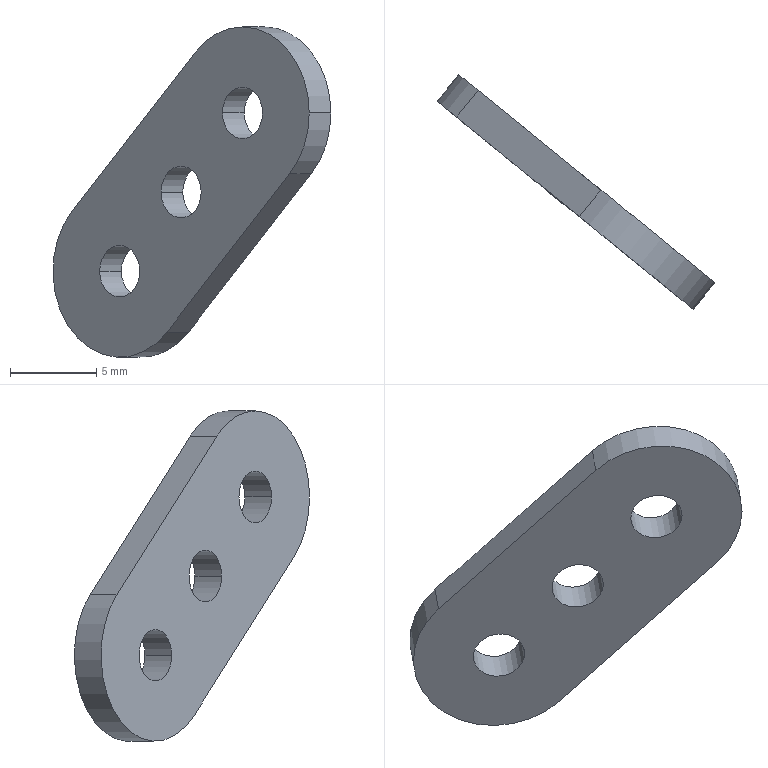Part | SolidWorks | features BaseBody 1 | 1 solid | 13 faces | box 16.152 x 13.661 x 19.192 mm | volume 374.668 mm3 | cylinder 9 | plane 4 | commonest cylinder face diameters 3 x6 10 x3
STEP:
#1=CARTESIAN_POINT('',(534.937,-167.759,275.623));
#2=VERTEX_POINT('',#1);
#3=CARTESIAN_POINT('',(536.073,-168.683,279.158));
#4=VERTEX_POINT('',#3);
#5=CARTESIAN_POINT('',(532.194,-165.528,279.158));
#6=DIRECTION('',(-0.6309,-0.7758,0.000000012));
#7=DIRECTION('',(0.7758,-0.6309,0.));
#8=AXIS2_PLACEMENT_3D('',#5,#6,#7);
#9=CIRCLE('',#8,5.);
#10=EDGE_CURVE('',#2,#4,#9,.T.);
#11=ORIENTED_EDGE('',*,*,#10,.T.);
#12=CARTESIAN_POINT('',(534.812,-170.235,279.158));
#13=VERTEX_POINT('',#12);
#14=CARTESIAN_POINT('',(536.073,-168.683,279.158));
#15=DIRECTION('',(-0.6309,-0.7758,0.000000012));
#16=VECTOR('',#15,1000.);
#17=LINE('',#14,#16);
#18=EDGE_CURVE('',#4,#13,#17,.T.);
#19=ORIENTED_EDGE('',*,*,#18,.T.);
#20=CARTESIAN_POINT('',(533.675,-169.311,275.623));
#21=VERTEX_POINT('',#20);
#22=CARTESIAN_POINT('',(530.932,-167.08,279.158));
#23=DIRECTION('',(0.6309,0.7758,-0.000000012));
#24=DIRECTION('',(0.7758,-0.6309,0.));
#25=AXIS2_PLACEMENT_3D('',#22,#23,#24);
#26=CIRCLE('',#25,5.);
#27=EDGE_CURVE('',#13,#21,#26,.T.);
#28=ORIENTED_EDGE('',*,*,#27,.T.);
#29=CARTESIAN_POINT('',(534.937,-167.759,275.623));
#30=DIRECTION('',(0.6309,0.7758,-0.000000012));
#31=VECTOR('',#30,1000.);
#32=LINE('',#29,#31);
#33=EDGE_CURVE('',#21,#2,#32,.T.);
#34=ORIENTED_EDGE('',*,*,#33,.T.);
#35=EDGE_LOOP('',(#11,#19,#28,#34));
#36=FACE_OUTER_BOUND('',#35,.T.);
#37=CARTESIAN_POINT('',(532.194,-165.528,279.158));
#38=DIRECTION('',(-0.6309,-0.7758,0.000000012));
#39=DIRECTION('',(0.7758,-0.6309,0.));
#40=AXIS2_PLACEMENT_3D('',#37,#38,#39);
#41=CYLINDRICAL_SURFACE('',#40,5.);
#42=ADVANCED_FACE('',(#36),#41,.T.);
#43=CARTESIAN_POINT('',(529.792,-163.575,274.562));
#44=VERTEX_POINT('',#43);
#45=CARTESIAN_POINT('',(527.465,-161.682,274.562));
#46=VERTEX_POINT('',#45);
#47=CARTESIAN_POINT('',(528.628,-162.628,274.562));
#48=DIRECTION('',(0.6309,0.7758,-0.000000012));
#49=DIRECTION('',(0.7758,-0.6309,0.));
#50=AXIS2_PLACEMENT_3D('',#47,#48,#49);
#51=CIRCLE('',#50,1.5);
#52=EDGE_CURVE('',#44,#46,#51,.T.);
#53=ORIENTED_EDGE('',*,*,#52,.T.);
#54=CARTESIAN_POINT('',(526.203,-163.234,274.562));
#55=VERTEX_POINT('',#54);
#56=CARTESIAN_POINT('',(526.203,-163.234,274.562));
#57=DIRECTION('',(-0.6309,-0.7758,0.000000012));
#58=VECTOR('',#57,1000.);
#59=LINE('',#56,#58);
#60=EDGE_CURVE('',#46,#55,#59,.T.);
#61=ORIENTED_EDGE('',*,*,#60,.T.);
#62=CARTESIAN_POINT('',(528.53,-165.127,274.562));
#63=VERTEX_POINT('',#62);
#64=CARTESIAN_POINT('',(527.366,-164.18,274.562));
#65=DIRECTION('',(0.6309,0.7758,-0.000000012));
#66=DIRECTION('',(0.7758,-0.6309,0.));
#67=AXIS2_PLACEMENT_3D('',#64,#65,#66);
#68=CIRCLE('',#67,1.5);
#69=EDGE_CURVE('',#63,#55,#68,.T.);
#70=ORIENTED_EDGE('',*,*,#69,.F.);
#71=CARTESIAN_POINT('',(528.53,-165.127,274.562));
#72=DIRECTION('',(-0.6309,-0.7758,0.000000012));
#73=VECTOR('',#72,1000.);
#74=LINE('',#71,#73);
#75=EDGE_CURVE('',#44,#63,#74,.T.);
#76=ORIENTED_EDGE('',*,*,#75,.F.);
#77=EDGE_LOOP('',(#53,#61,#70,#76));
#78=FACE_OUTER_BOUND('',#77,.T.);
#79=CARTESIAN_POINT('',(527.366,-164.18,274.562));
#80=DIRECTION('',(-0.6309,-0.7758,0.000000012));
#81=DIRECTION('',(0.7758,-0.6309,0.));
#82=AXIS2_PLACEMENT_3D('',#79,#80,#81);
#83=CYLINDRICAL_SURFACE('',#82,1.5);
#84=ADVANCED_FACE('',(#78),#83,.F.);
#85=CARTESIAN_POINT('',(526.226,-160.675,269.966));
#86=VERTEX_POINT('',#85);
#87=CARTESIAN_POINT('',(523.899,-158.782,269.966));
#88=VERTEX_POINT('',#87);
#89=CARTESIAN_POINT('',(525.062,-159.729,269.966));
#90=DIRECTION('',(0.6309,0.7758,-0.000000012));
#91=DIRECTION('',(0.7758,-0.6309,0.));
#92=AXIS2_PLACEMENT_3D('',#89,#90,#91);
#93=CIRCLE('',#92,1.5);
#94=EDGE_CURVE('',#86,#88,#93,.T.);
#95=ORIENTED_EDGE('',*,*,#94,.T.);
#96=CARTESIAN_POINT('',(522.637,-160.334,269.966));
#97=VERTEX_POINT('',#96);
#98=CARTESIAN_POINT('',(522.637,-160.334,269.966));
#99=DIRECTION('',(-0.6309,-0.7758,0.000000012));
#100=VECTOR('',#99,1000.);
#101=LINE('',#98,#100);
#102=EDGE_CURVE('',#88,#97,#101,.T.);
#103=ORIENTED_EDGE('',*,*,#102,.T.);
#104=CARTESIAN_POINT('',(524.964,-162.227,269.966));
#105=VERTEX_POINT('',#104);
#106=CARTESIAN_POINT('',(523.801,-161.28,269.966));
#107=DIRECTION('',(0.6309,0.7758,-0.000000012));
#108=DIRECTION('',(0.7758,-0.6309,0.));
#109=AXIS2_PLACEMENT_3D('',#106,#107,#108);
#110=CIRCLE('',#109,1.5);
#111=EDGE_CURVE('',#105,#97,#110,.T.);
#112=ORIENTED_EDGE('',*,*,#111,.F.);
#113=CARTESIAN_POINT('',(524.964,-162.227,269.966));
#114=DIRECTION('',(-0.6309,-0.7758,0.000000012));
#115=VECTOR('',#114,1000.);
#116=LINE('',#113,#115);
#117=EDGE_CURVE('',#86,#105,#116,.T.);
#118=ORIENTED_EDGE('',*,*,#117,.F.);
#119=EDGE_LOOP('',(#95,#103,#112,#118));
#120=FACE_OUTER_BOUND('',#119,.T.);
#121=CARTESIAN_POINT('',(523.801,-161.28,269.966));
#122=DIRECTION('',(-0.6309,-0.7758,0.000000012));
#123=DIRECTION('',(0.7758,-0.6309,0.));
#124=AXIS2_PLACEMENT_3D('',#121,#122,#123);
#125=CYLINDRICAL_SURFACE('',#124,1.5);
#126=ADVANCED_FACE('',(#120),#125,.F.);
#127=CARTESIAN_POINT('',(533.358,-166.475,279.158));
#128=VERTEX_POINT('',#127);
#129=CARTESIAN_POINT('',(531.03,-164.582,279.158));
#130=VERTEX_POINT('',#129);
#131=CARTESIAN_POINT('',(532.194,-165.528,279.158));
#132=DIRECTION('',(0.6309,0.7758,-0.000000012));
#133=DIRECTION('',(0.7758,-0.6309,0.));
#134=AXIS2_PLACEMENT_3D('',#131,#132,#133);
#135=CIRCLE('',#134,1.5);
#136=EDGE_CURVE('',#128,#130,#135,.T.);
#137=ORIENTED_EDGE('',*,*,#136,.T.);
#138=CARTESIAN_POINT('',(529.769,-166.134,279.158));
#139=VERTEX_POINT('',#138);
#140=CARTESIAN_POINT('',(529.769,-166.134,279.158));
#141=DIRECTION('',(-0.6309,-0.7758,0.000000012));
#142=VECTOR('',#141,1000.);
#143=LINE('',#140,#142);
#144=EDGE_CURVE('',#130,#139,#143,.T.);
#145=ORIENTED_EDGE('',*,*,#144,.T.);
#146=CARTESIAN_POINT('',(532.096,-168.026,279.158));
#147=VERTEX_POINT('',#146);
#148=CARTESIAN_POINT('',(530.932,-167.08,279.158));
#149=DIRECTION('',(0.6309,0.7758,-0.000000012));
#150=DIRECTION('',(0.7758,-0.6309,0.));
#151=AXIS2_PLACEMENT_3D('',#148,#149,#150);
#152=CIRCLE('',#151,1.5);
#153=EDGE_CURVE('',#147,#139,#152,.T.);
#154=ORIENTED_EDGE('',*,*,#153,.F.);
#155=CARTESIAN_POINT('',(532.096,-168.026,279.158));
#156=DIRECTION('',(-0.6309,-0.7758,0.000000012));
#157=VECTOR('',#156,1000.);
#158=LINE('',#155,#157);
#159=EDGE_CURVE('',#128,#147,#158,.T.);
#160=ORIENTED_EDGE('',*,*,#159,.F.);
#161=EDGE_LOOP('',(#137,#145,#154,#160));
#162=FACE_OUTER_BOUND('',#161,.T.);
#163=CARTESIAN_POINT('',(530.932,-167.08,279.158));
#164=DIRECTION('',(-0.6309,-0.7758,0.000000012));
#165=DIRECTION('',(0.7758,-0.6309,0.));
#166=AXIS2_PLACEMENT_3D('',#163,#164,#165);
#167=CYLINDRICAL_SURFACE('',#166,1.5);
#168=ADVANCED_FACE('',(#162),#167,.F.);
#169=CARTESIAN_POINT('',(527.805,-161.959,266.431));
#170=VERTEX_POINT('',#169);
#171=CARTESIAN_POINT('',(527.805,-161.959,266.431));
#172=DIRECTION('',(0.5486,-0.4461,0.7071));
#173=VECTOR('',#172,1000.);
#174=LINE('',#171,#173);
#175=EDGE_CURVE('',#170,#2,#174,.T.);
#176=ORIENTED_EDGE('',*,*,#175,.F.);
#177=CARTESIAN_POINT('',(522.319,-157.498,273.502));
#178=VERTEX_POINT('',#177);
#179=CARTESIAN_POINT('',(525.062,-159.729,269.966));
#180=DIRECTION('',(-0.6309,-0.7758,0.000000012));
#181=DIRECTION('',(0.7758,-0.6309,0.));
#182=AXIS2_PLACEMENT_3D('',#179,#180,#181);
#183=CIRCLE('',#182,5.);
#184=EDGE_CURVE('',#178,#170,#183,.T.);
#185=ORIENTED_EDGE('',*,*,#184,.F.);
#186=CARTESIAN_POINT('',(529.451,-163.298,282.694));
#187=VERTEX_POINT('',#186);
#188=CARTESIAN_POINT('',(529.451,-163.298,282.694));
#189=DIRECTION('',(-0.5486,0.4461,-0.7071));
#190=VECTOR('',#189,1000.);
#191=LINE('',#188,#190);
#192=EDGE_CURVE('',#187,#178,#191,.T.);
#193=ORIENTED_EDGE('',*,*,#192,.F.);
#194=CARTESIAN_POINT('',(532.194,-165.528,279.158));
#195=DIRECTION('',(-0.6309,-0.7758,0.000000012));
#196=DIRECTION('',(0.7758,-0.6309,0.));
#197=AXIS2_PLACEMENT_3D('',#194,#195,#196);
#198=CIRCLE('',#197,5.);
#199=EDGE_CURVE('',#4,#187,#198,.T.);
#200=ORIENTED_EDGE('',*,*,#199,.F.);
#201=ORIENTED_EDGE('',*,*,#10,.F.);
#202=EDGE_LOOP('',(#176,#185,#193,#200,#201));
#203=FACE_OUTER_BOUND('',#202,.T.);
#204=ORIENTED_EDGE('',*,*,#52,.F.);
#205=CARTESIAN_POINT('',(528.628,-162.628,274.562));
#206=DIRECTION('',(0.6309,0.7758,-0.000000012));
#207=DIRECTION('',(0.7758,-0.6309,0.));
#208=AXIS2_PLACEMENT_3D('',#205,#206,#207);
#209=CIRCLE('',#208,1.5);
#210=EDGE_CURVE('',#46,#44,#209,.T.);
#211=ORIENTED_EDGE('',*,*,#210,.F.);
#212=EDGE_LOOP('',(#204,#211));
#213=FACE_BOUND('',#212,.T.);
#214=ORIENTED_EDGE('',*,*,#94,.F.);
#215=CARTESIAN_POINT('',(525.062,-159.729,269.966));
#216=DIRECTION('',(0.6309,0.7758,-0.000000012));
#217=DIRECTION('',(0.7758,-0.6309,0.));
#218=AXIS2_PLACEMENT_3D('',#215,#216,#217);
#219=CIRCLE('',#218,1.5);
#220=EDGE_CURVE('',#88,#86,#219,.T.);
#221=ORIENTED_EDGE('',*,*,#220,.F.);
#222=EDGE_LOOP('',(#214,#221));
#223=FACE_BOUND('',#222,.T.);
#224=ORIENTED_EDGE('',*,*,#136,.F.);
#225=CARTESIAN_POINT('',(532.194,-165.528,279.158));
#226=DIRECTION('',(0.6309,0.7758,-0.000000012));
#227=DIRECTION('',(0.7758,-0.6309,0.));
#228=AXIS2_PLACEMENT_3D('',#225,#226,#227);
#229=CIRCLE('',#228,1.5);
#230=EDGE_CURVE('',#130,#128,#229,.T.);
#231=ORIENTED_EDGE('',*,*,#230,.F.);
#232=EDGE_LOOP('',(#224,#231));
#233=FACE_BOUND('',#232,.T.);
#234=CARTESIAN_POINT('',(528.628,-162.628,274.562));
#235=DIRECTION('',(-0.6309,-0.7758,0.000000012));
#236=DIRECTION('',(0.7758,-0.6309,0.));
#237=AXIS2_PLACEMENT_3D('',#234,#235,#236);
#238=PLANE('',#237);
#239=ADVANCED_FACE('',(#203,#213,#223,#233),#238,.F.);
#240=ORIENTED_EDGE('',*,*,#18,.F.);
#241=ORIENTED_EDGE('',*,*,#199,.T.);
#242=CARTESIAN_POINT('',(528.189,-164.849,282.694));
#243=VERTEX_POINT('',#242);
#244=CARTESIAN_POINT('',(528.189,-164.849,282.694));
#245=DIRECTION('',(0.6309,0.7758,-0.000000012));
#246=VECTOR('',#245,1000.);
#247=LINE('',#244,#246);
#248=EDGE_CURVE('',#243,#187,#247,.T.);
#249=ORIENTED_EDGE('',*,*,#248,.F.);
#250=CARTESIAN_POINT('',(530.932,-167.08,279.158));
#251=DIRECTION('',(0.6309,0.7758,-0.000000012));
#252=DIRECTION('',(0.7758,-0.6309,0.));
#253=AXIS2_PLACEMENT_3D('',#250,#251,#252);
#254=CIRCLE('',#253,5.);
#255=EDGE_CURVE('',#243,#13,#254,.T.);
#256=ORIENTED_EDGE('',*,*,#255,.T.);
#257=EDGE_LOOP('',(#240,#241,#249,#256));
#258=FACE_OUTER_BOUND('',#257,.T.);
#259=CARTESIAN_POINT('',(532.194,-165.528,279.158));
#260=DIRECTION('',(-0.6309,-0.7758,0.000000012));
#261=DIRECTION('',(0.7758,-0.6309,0.));
#262=AXIS2_PLACEMENT_3D('',#259,#260,#261);
#263=CYLINDRICAL_SURFACE('',#262,5.);
#264=ADVANCED_FACE('',(#258),#263,.T.);
#265=CARTESIAN_POINT('',(526.544,-163.511,266.431));
#266=VERTEX_POINT('',#265);
#267=CARTESIAN_POINT('',(526.544,-163.511,266.431));
#268=DIRECTION('',(0.6309,0.7758,-0.000000012));
#269=VECTOR('',#268,1000.);
#270=LINE('',#267,#269);
#271=EDGE_CURVE('',#266,#170,#270,.T.);
#272=ORIENTED_EDGE('',*,*,#271,.T.);
#273=ORIENTED_EDGE('',*,*,#175,.T.);
#274=ORIENTED_EDGE('',*,*,#33,.F.);
#275=CARTESIAN_POINT('',(533.675,-169.311,275.623));
#276=DIRECTION('',(-0.5486,0.4461,-0.7071));
#277=VECTOR('',#276,1000.);
#278=LINE('',#275,#277);
#279=EDGE_CURVE('',#21,#266,#278,.T.);
#280=ORIENTED_EDGE('',*,*,#279,.T.);
#281=EDGE_LOOP('',(#272,#273,#274,#280));
#282=FACE_OUTER_BOUND('',#281,.T.);
#283=CARTESIAN_POINT('',(537.68,-169.99,279.158));
#284=DIRECTION('',(0.5486,-0.4461,-0.7071));
#285=DIRECTION('',(-0.7901,0.,-0.613));
#286=AXIS2_PLACEMENT_3D('',#283,#284,#285);
#287=PLANE('',#286);
#288=ADVANCED_FACE('',(#282),#287,.T.);
#289=ORIENTED_EDGE('',*,*,#271,.F.);
#290=CARTESIAN_POINT('',(521.058,-159.05,273.502));
#291=VERTEX_POINT('',#290);
#292=CARTESIAN_POINT('',(523.801,-161.28,269.966));
#293=DIRECTION('',(0.6309,0.7758,-0.000000012));
#294=DIRECTION('',(0.7758,-0.6309,0.));
#295=AXIS2_PLACEMENT_3D('',#292,#293,#294);
#296=CIRCLE('',#295,5.);
#297=EDGE_CURVE('',#266,#291,#296,.T.);
#298=ORIENTED_EDGE('',*,*,#297,.T.);
#299=CARTESIAN_POINT('',(522.319,-157.498,273.502));
#300=DIRECTION('',(0.6309,0.7758,-0.000000012));
#301=VECTOR('',#300,1000.);
#302=LINE('',#299,#301);
#303=EDGE_CURVE('',#291,#178,#302,.T.);
#304=ORIENTED_EDGE('',*,*,#303,.T.);
#305=ORIENTED_EDGE('',*,*,#184,.T.);
#306=EDGE_LOOP('',(#289,#298,#304,#305));
#307=FACE_OUTER_BOUND('',#306,.T.);
#308=CARTESIAN_POINT('',(525.062,-159.729,269.966));
#309=DIRECTION('',(-0.6309,-0.7758,0.000000012));
#310=DIRECTION('',(0.7758,-0.6309,0.));
#311=AXIS2_PLACEMENT_3D('',#308,#309,#310);
#312=CYLINDRICAL_SURFACE('',#311,5.);
#313=ADVANCED_FACE('',(#307),#312,.T.);
#314=ORIENTED_EDGE('',*,*,#303,.F.);
#315=CARTESIAN_POINT('',(521.058,-159.05,273.502));
#316=DIRECTION('',(0.5486,-0.4461,0.7071));
#317=VECTOR('',#316,1000.);
#318=LINE('',#315,#317);
#319=EDGE_CURVE('',#291,#243,#318,.T.);
#320=ORIENTED_EDGE('',*,*,#319,.T.);
#321=ORIENTED_EDGE('',*,*,#248,.T.);
#322=ORIENTED_EDGE('',*,*,#192,.T.);
#323=EDGE_LOOP('',(#314,#320,#321,#322));
#324=FACE_OUTER_BOUND('',#323,.T.);
#325=CARTESIAN_POINT('',(519.576,-155.267,269.966));
#326=DIRECTION('',(-0.5486,0.4461,0.7071));
#327=DIRECTION('',(0.7901,0.,0.613));
#328=AXIS2_PLACEMENT_3D('',#325,#326,#327);
#329=PLANE('',#328);
#330=ADVANCED_FACE('',(#324),#329,.T.);
#331=ORIENTED_EDGE('',*,*,#60,.F.);
#332=ORIENTED_EDGE('',*,*,#210,.T.);
#333=ORIENTED_EDGE('',*,*,#75,.T.);
#334=CARTESIAN_POINT('',(527.366,-164.18,274.562));
#335=DIRECTION('',(0.6309,0.7758,-0.000000012));
#336=DIRECTION('',(0.7758,-0.6309,0.));
#337=AXIS2_PLACEMENT_3D('',#334,#335,#336);
#338=CIRCLE('',#337,1.5);
#339=EDGE_CURVE('',#55,#63,#338,.T.);
#340=ORIENTED_EDGE('',*,*,#339,.F.);
#341=EDGE_LOOP('',(#331,#332,#333,#340));
#342=FACE_OUTER_BOUND('',#341,.T.);
#343=CARTESIAN_POINT('',(527.366,-164.18,274.562));
#344=DIRECTION('',(-0.6309,-0.7758,0.000000012));
#345=DIRECTION('',(0.7758,-0.6309,0.));
#346=AXIS2_PLACEMENT_3D('',#343,#344,#345);
#347=CYLINDRICAL_SURFACE('',#346,1.5);
#348=ADVANCED_FACE('',(#342),#347,.F.);
#349=ORIENTED_EDGE('',*,*,#102,.F.);
#350=ORIENTED_EDGE('',*,*,#220,.T.);
#351=ORIENTED_EDGE('',*,*,#117,.T.);
#352=CARTESIAN_POINT('',(523.801,-161.28,269.966));
#353=DIRECTION('',(0.6309,0.7758,-0.000000012));
#354=DIRECTION('',(0.7758,-0.6309,0.));
#355=AXIS2_PLACEMENT_3D('',#352,#353,#354);
#356=CIRCLE('',#355,1.5);
#357=EDGE_CURVE('',#97,#105,#356,.T.);
#358=ORIENTED_EDGE('',*,*,#357,.F.);
#359=EDGE_LOOP('',(#349,#350,#351,#358));
#360=FACE_OUTER_BOUND('',#359,.T.);
#361=CARTESIAN_POINT('',(523.801,-161.28,269.966));
#362=DIRECTION('',(-0.6309,-0.7758,0.000000012));
#363=DIRECTION('',(0.7758,-0.6309,0.));
#364=AXIS2_PLACEMENT_3D('',#361,#362,#363);
#365=CYLINDRICAL_SURFACE('',#364,1.5);
#366=ADVANCED_FACE('',(#360),#365,.F.);
#367=ORIENTED_EDGE('',*,*,#144,.F.);
#368=ORIENTED_EDGE('',*,*,#230,.T.);
#369=ORIENTED_EDGE('',*,*,#159,.T.);
#370=CARTESIAN_POINT('',(530.932,-167.08,279.158));
#371=DIRECTION('',(0.6309,0.7758,-0.000000012));
#372=DIRECTION('',(0.7758,-0.6309,0.));
#373=AXIS2_PLACEMENT_3D('',#370,#371,#372);
#374=CIRCLE('',#373,1.5);
#375=EDGE_CURVE('',#139,#147,#374,.T.);
#376=ORIENTED_EDGE('',*,*,#375,.F.);
#377=EDGE_LOOP('',(#367,#368,#369,#376));
#378=FACE_OUTER_BOUND('',#377,.T.);
#379=CARTESIAN_POINT('',(530.932,-167.08,279.158));
#380=DIRECTION('',(-0.6309,-0.7758,0.000000012));
#381=DIRECTION('',(0.7758,-0.6309,0.));
#382=AXIS2_PLACEMENT_3D('',#379,#380,#381);
#383=CYLINDRICAL_SURFACE('',#382,1.5);
#384=ADVANCED_FACE('',(#378),#383,.F.);
#385=ORIENTED_EDGE('',*,*,#279,.F.);
#386=ORIENTED_EDGE('',*,*,#27,.F.);
#387=ORIENTED_EDGE('',*,*,#255,.F.);
#388=ORIENTED_EDGE('',*,*,#319,.F.);
#389=ORIENTED_EDGE('',*,*,#297,.F.);
#390=EDGE_LOOP('',(#385,#386,#387,#388,#389));
#391=FACE_OUTER_BOUND('',#390,.T.);
#392=ORIENTED_EDGE('',*,*,#69,.T.);
#393=ORIENTED_EDGE('',*,*,#339,.T.);
#394=EDGE_LOOP('',(#392,#393));
#395=FACE_BOUND('',#394,.T.);
#396=ORIENTED_EDGE('',*,*,#111,.T.);
#397=ORIENTED_EDGE('',*,*,#357,.T.);
#398=EDGE_LOOP('',(#396,#397));
#399=FACE_BOUND('',#398,.T.);
#400=ORIENTED_EDGE('',*,*,#153,.T.);
#401=ORIENTED_EDGE('',*,*,#375,.T.);
#402=EDGE_LOOP('',(#400,#401));
#403=FACE_BOUND('',#402,.T.);
#404=CARTESIAN_POINT('',(527.366,-164.18,274.562));
#405=DIRECTION('',(-0.6309,-0.7758,0.000000012));
#406=DIRECTION('',(0.7758,-0.6309,0.));
#407=AXIS2_PLACEMENT_3D('',#404,#405,#406);
#408=PLANE('',#407);
#409=ADVANCED_FACE('',(#391,#395,#399,#403),#408,.T.);
#410=CLOSED_SHELL('',(#42,#84,#126,#168,#239,#264,#288,#313,#330,#348,#366,#384,#409));
#411=MANIFOLD_SOLID_BREP('',#410);
#412=CARTESIAN_POINT('',(0.,0.,0.));
#413=DIRECTION('',(0.,0.,1.));
#414=DIRECTION('',(1.,0.,0.));
#415=AXIS2_PLACEMENT_3D('',#412,#413,#414);
#416=(LENGTH_UNIT()NAMED_UNIT(*)SI_UNIT(.MILLI.,.METRE.));
#417=UNCERTAINTY_MEASURE_WITH_UNIT(LENGTH_MEASURE(0.00001),#416,'','');
#418=(NAMED_UNIT(*)PLANE_ANGLE_UNIT()SI_UNIT($,.RADIAN.));
#419=(NAMED_UNIT(*)SI_UNIT($,.STERADIAN.)SOLID_ANGLE_UNIT());
#420=(GEOMETRIC_REPRESENTATION_CONTEXT(3)GLOBAL_UNCERTAINTY_ASSIGNED_CONTEXT((#417))GLOBAL_UNIT_ASSIGNED_CONTEXT((#416,#418,#419))REPRESENTATION_CONTEXT('',''));
#421=ADVANCED_BREP_SHAPE_REPRESENTATION('',(#411,#415),#420);